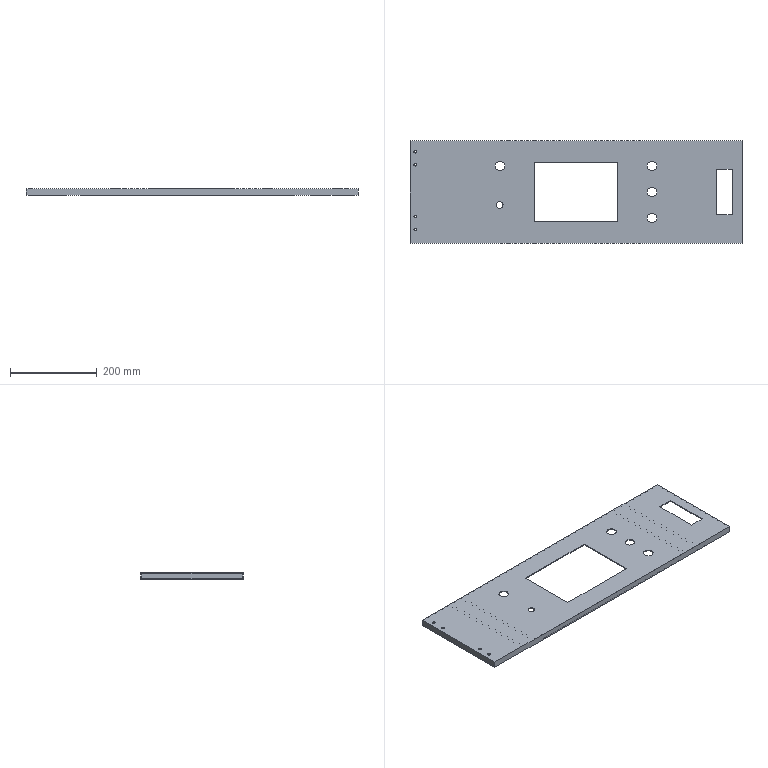Part | STEP file | Front upper door | 1 solid | 84 faces | box 767 x 237 x 15 mm | volume 445389 mm3 | plane 62 | cylinder 22 | commonest cylinder face diameters 6.2 x12 22.2 x8 15 x2